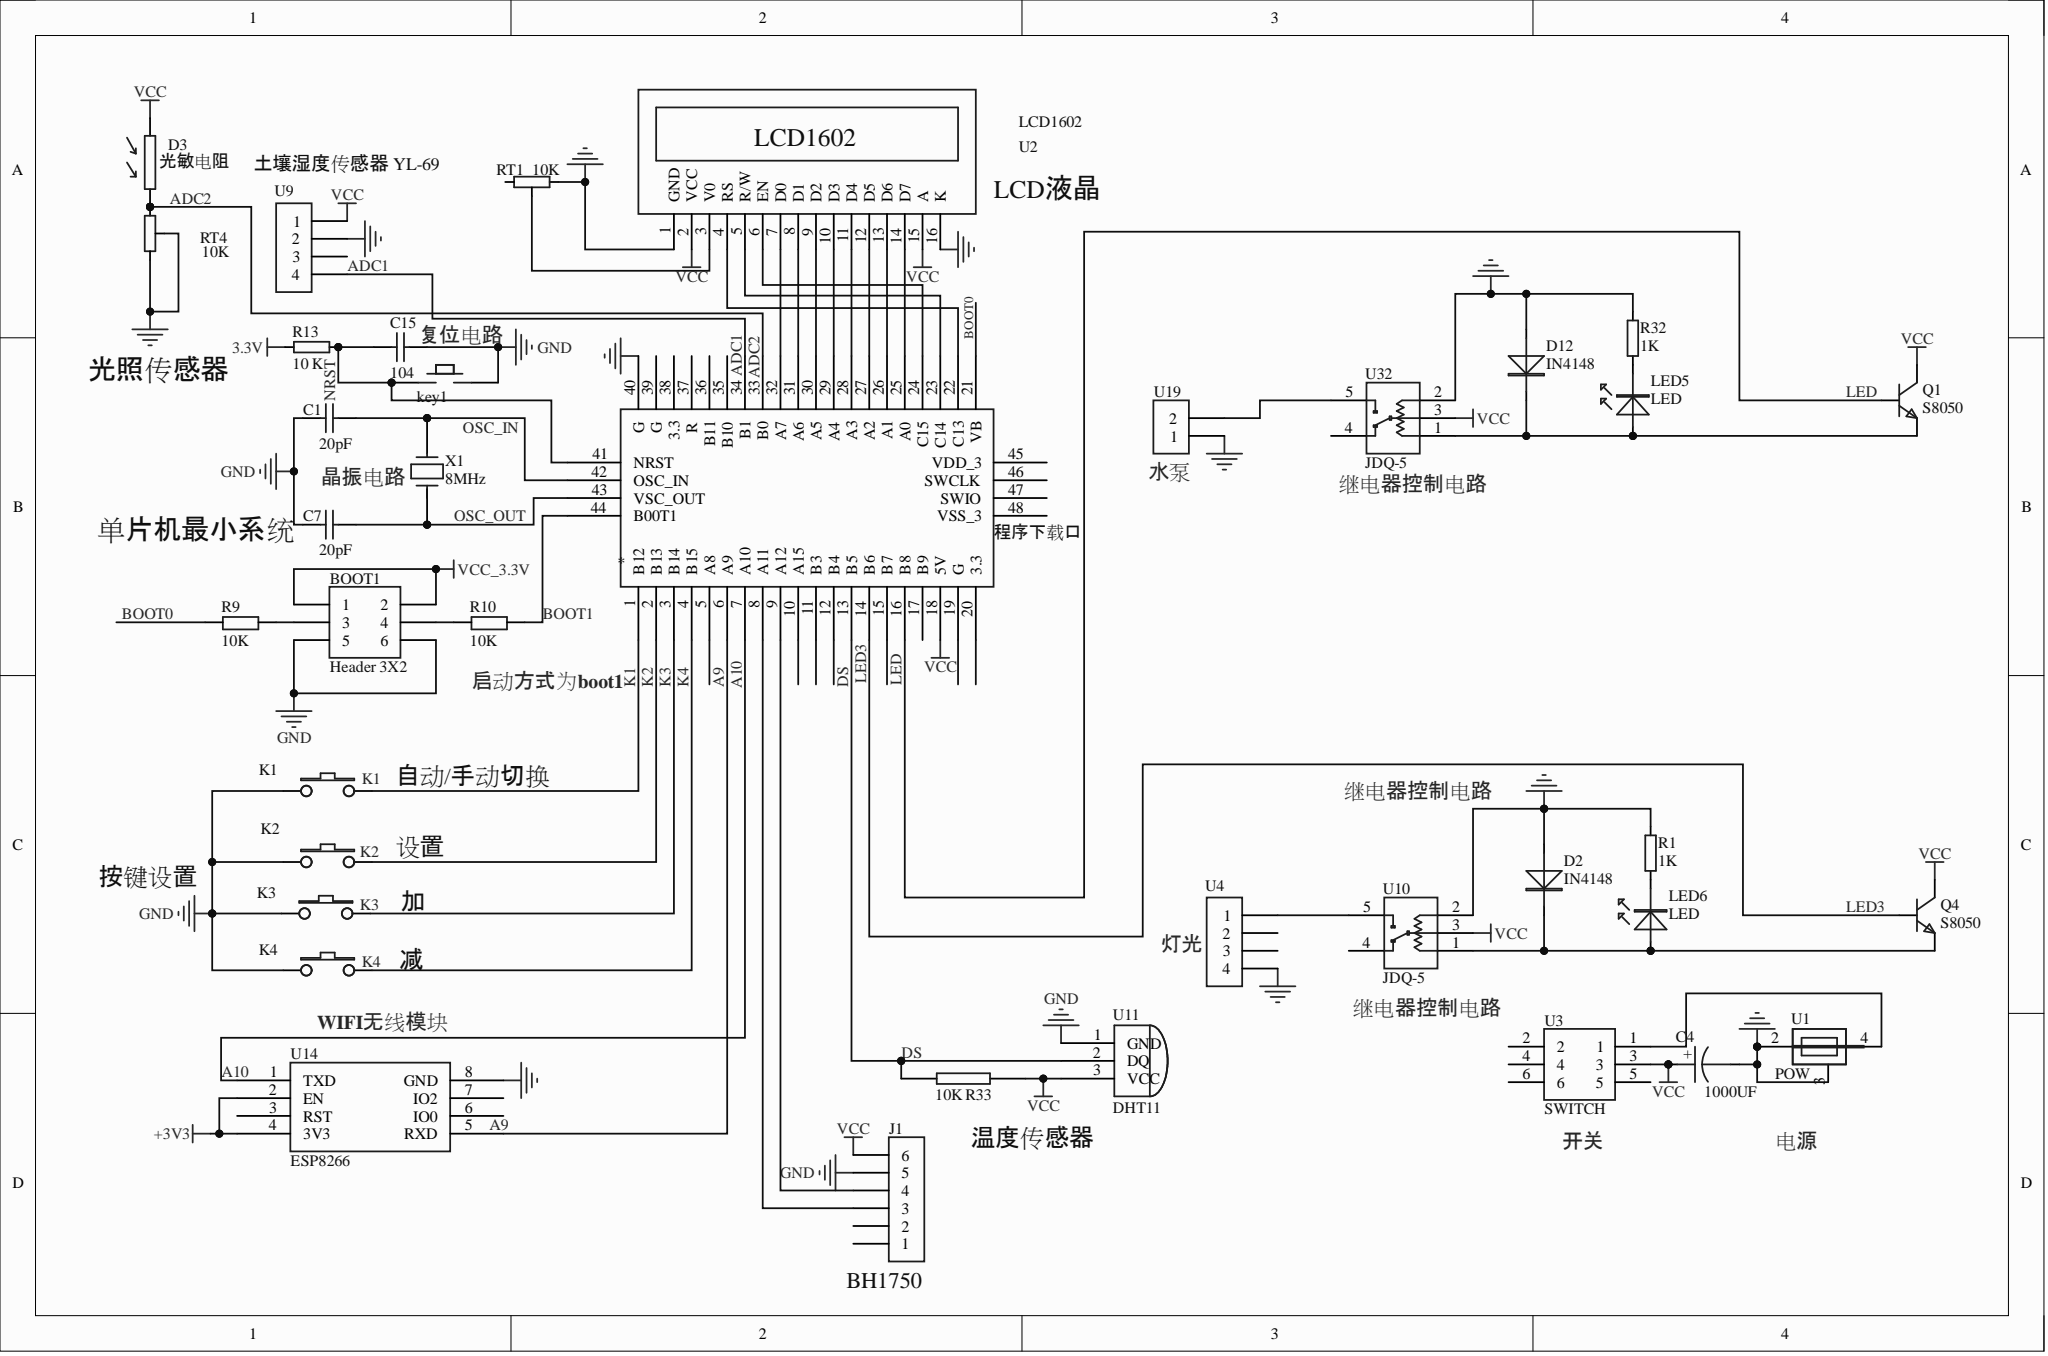Circuit board | Altium Designer | 38 parts | 43 nets
Bill of materials:
Comment,Description,Designator,Footprint,LibRef,Quantity
"","","","LQFP-48_L7.0-W7.0-P0.50-LS9.0-BL","","1"
"Header 3X2","Header, 3-Pin, Dual row","BOOT1","HDR-TH_6P-P2.54-V-F-R2-C3-S2.54","Header 3X2","1"
"20pF","Capacitor","C1, C7","C0603","20pF","2"
"1000UF","","C4","CAP-TH_BD8.0-P3.50-D0.6-FD_1","1000UF","1"
"104","Capacitor","C15","C0603","104","1"
"IN4148","","D2, D12","SOD-323_L1.8-W1.3-LS2.5-RD","IN4148","2"
"光敏电阻","","D3","RES-TH_L8.0-W4.4-P4.50-D0.6-S2.0","光敏电阻","1"
"","","J1","HDR-TH_6P-P2.54-V-F","J?","1"
"","","K1, K2, K3, K4","Key_SMD_3x4x2","K1, K2, K3, K4","4"
"KEY_M","","key1","Key_SMD_3x4x2","KEY_M","1"
"LED","","LED5, LED6","LED0603","LED","2"
"S8050","","Q1, Q4","S8050_SOT-23","S8050","2"
"1K","","R1, R32","R0603","1K","2"
"10K","","R9, R10, R33","R0603","10K_1, 10K_2","3"
"10 K","","R13","R0603","10 K","1"
"10K","","RT1, RT4","R_3296","10K","2"
"POW","","U1","DC-2.0","POW","1"
"LCD1602","","U2","LCD1602","LCD1602","1"
"SWITCH","","U3","SW-TH_6P-L5.8-W5.8-P2.00-LS4.5-TR","SWITCH","1"
"","Connector","U4, U9","HDR-TH_4P-P2.54-V-F","U9","2"
"JDQ-5","","U10, U32","RELAY-TH_FTR-K1CK024W","JDQ-5","2"
"DHT11","","U11","HDR-TH_3P-P2.54-V-F","DHT11","1"
"ESP8266","","U14","WIFIM-TH_8P-L24.7-W14.4-P2.54","ESP8266","1"
"","","U19","CONN-TH_XH2.54-2P","U19","1"
"8MHz","Crystal","X1","CRYSTAL-SMD_L3.2-W2.5_3225-8MHZ","8MHz","1"
Netlist (Protel format):
[
*
LQFP-48_L7.0-W7.0-P0.50-LS9.0-BL
程序下载口



]
[
BOOT1
HDR-TH_6P-P2.54-V-F-R2-C3-S2.54
Header 3X2



]
[
C1
C0603
20pF



]
[
C4
CAP-TH_BD8.0-P3.50-D0.6-FD_1
1000UF



]
[
C7
C0603
20pF



]
[
C15
C0603
104



]
[
D2
SOD-323_L1.8-W1.3-LS2.5-RD
IN4148



]
[
D3
RES-TH_L8.0-W4.4-P4.50-D0.6-S2.0
光敏电阻



]
[
D12
SOD-323_L1.8-W1.3-LS2.5-RD
IN4148



]
[
J1
HDR-TH_6P-P2.54-V-F




]
[
K1
Key_SMD_3x4x2




]
[
K2
Key_SMD_3x4x2




]
[
K3
Key_SMD_3x4x2




]
[
K4
Key_SMD_3x4x2




]
[
key1
Key_SMD_3x4x2
KEY_M



]
[
LED5
LED0603
LED



]
[
LED6
LED0603
LED



]
[
Q1
S8050_SOT-23
S8050



]
[
Q4
S8050_SOT-23
S8050



]
[
R1
R0603
1K



]
[
R9
R0603
10K



]
[
R10
R0603
10K



]
[
R13
R0603
10 K



]
[
R32
R0603
1K



]
[
R33
R0603
10K



]
[
RT1
R_3296
10K



]
[
RT4
R_3296
10K



]
[
U1
DC-2.0
POW



]
[
U2
LCD1602
LCD1602



]
[
U3
SW-TH_6P-L5.8-W5.8-P2.00-LS4.5-TR
SWITCH



]
[
U4
HDR-TH_4P-P2.54-V-F




]
[
U9
HDR-TH_4P-P2.54-V-F




]
[
U10
RELAY-TH_FTR-K1CK024W
JDQ-5



]
[
U11
HDR-TH_3P-P2.54-V-F
DHT11



]
[
U14
WIFIM-TH_8P-L24.7-W14.4-P2.54
ESP8266



]
[
U19
CONN-TH_XH2.54-2P




]
[
U32
RELAY-TH_FTR-K1CK024W
JDQ-5



]
[
X1
CRYSTAL-SMD_L3.2-W2.5_3225-8MHZ
8MHz



]
(
VCC_3.3V
BOOT1-1
BOOT1-2
)
(
VCC
*-18
C4-1
D3-1
J1-6
Q1-3
Q4-3
R33-2
U2-2
U2-15
U3-3
U9-1
U10-3
U11-3
U32-3
)
(
OSC_OUT
*-43
C7-2
X1-1
)
(
NetU19_2
U19-2
U32-5
)
(
NetU4_1
U4-1
U10-5
)
(
NetU1_4
U1-4
U3-1
)
(
NetRT1_2
RT1-2
U2-3
)
(
NetLED6_2
LED6-2
R1-2
)
(
NetLED5_2
LED5-2
R32-2
)
(
NetD12_2
D12-2
LED5-1
Q1-2
U32-1
)
(
NetD2_2
D2-2
LED6-1
Q4-2
U10-1
)
(
NetBOOT1_4
BOOT1-4
R10-1
)
(
NetBOOT1_3
BOOT1-3
R9-2
)
(
Net*_42
*-42
C1-2
X1-2
)
(
Net*_41
*-41
C15-2
key1-1
R13-2
)
(
Net*_32
*-32
U2-7
)
(
Net*_31
*-31
U2-8
)
(
Net*_30
*-30
U2-9
)
(
Net*_29
*-29
U2-10
)
(
Net*_28
*-28
U2-11
)
(
Net*_27
*-27
U2-12
)
(
Net*_26
*-26
U2-13
)
(
Net*_25
*-25
U2-14
)
(
Net*_24
*-24
U2-6
)
(
Net*_23
*-23
U2-5
)
(
Net*_22
*-22
U2-4
)
(
Net*_9
*-9
J1-4
)
(
Net*_8
*-8
J1-3
)
(
LED3
*-14
Q4-1
)
(
LED
*-16
Q1-1
)
(
K4
*-4
K4-2
)
(
K3
*-3
K3-2
)
(
K2
*-2
K2-2
)
(
K1
*-1
K1-2
)
(
GND
*-40
BOOT1-5
BOOT1-6
C1-1
C4-2
C7-1
C15-1
D2-1
D12-1
J1-5
K1-1
K2-1
K3-1
K4-1
key1-2
R1-1
R32-1
RT1-3
RT4-1
RT4-2
U1-2
U1-3
U2-1
U2-16
U4-4
U9-2
U10-2
U11-1
U14-8
U19-1
U32-2
)
(
DS
*-13
R33-1
U11-2
)
(
BOOT1
*-44
R10-2
)
(
BOOT0
*-21
R9-1
)
(
ADC2
*-33
D3-2
RT4-3
)
(
ADC1
*-34
U9-4
)
(
A10
*-7
U14-1
)
(
A9
*-6
U14-5
)
(
+3V3
U14-2
U14-4
)